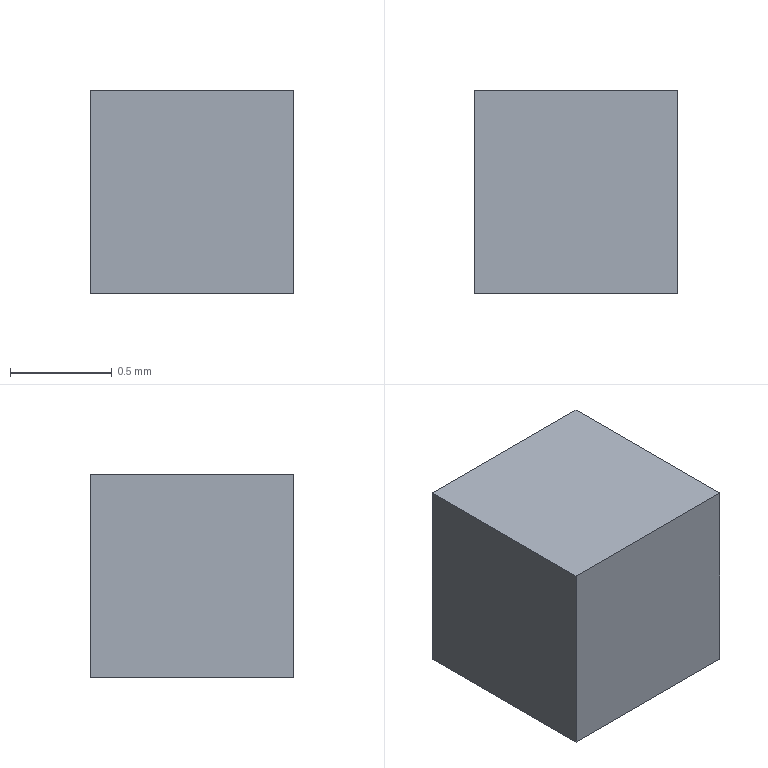Part | Creo | 1 solid | 6 faces | box 1 x 1 x 1 mm | volume 1 mm3 | plane 6
STEP:
#1=CARTESIAN_POINT('',(0.,0.,0.));
#2=DIRECTION('',(0.,0.,1.));
#3=DIRECTION('',(1.,0.,0.));
#4=AXIS2_PLACEMENT_3D('',#1,#2,#3);
#5=CARTESIAN_POINT('',(-0.5,-0.5,0.));
#6=VERTEX_POINT('',#5);
#7=CARTESIAN_POINT('',(0.5,-0.5,0.));
#8=VERTEX_POINT('',#7);
#9=CARTESIAN_POINT('',(-0.5,-0.5,0.));
#10=DIRECTION('',(1.,0.,0.));
#11=VECTOR('',#10,1.);
#12=LINE('',#9,#11);
#13=EDGE_CURVE('',#6,#8,#12,.T.);
#14=ORIENTED_EDGE('',*,*,#13,.T.);
#15=CARTESIAN_POINT('',(0.5,0.5,0.));
#16=VERTEX_POINT('',#15);
#17=CARTESIAN_POINT('',(0.5,-0.5,0.));
#18=DIRECTION('',(0.,1.,0.));
#19=VECTOR('',#18,1.);
#20=LINE('',#17,#19);
#21=EDGE_CURVE('',#8,#16,#20,.T.);
#22=ORIENTED_EDGE('',*,*,#21,.T.);
#23=CARTESIAN_POINT('',(-0.5,0.5,0.));
#24=VERTEX_POINT('',#23);
#25=CARTESIAN_POINT('',(0.5,0.5,0.));
#26=DIRECTION('',(-1.,0.,0.));
#27=VECTOR('',#26,1.);
#28=LINE('',#25,#27);
#29=EDGE_CURVE('',#16,#24,#28,.T.);
#30=ORIENTED_EDGE('',*,*,#29,.T.);
#31=CARTESIAN_POINT('',(-0.5,0.5,0.));
#32=DIRECTION('',(0.,-1.,0.));
#33=VECTOR('',#32,1.);
#34=LINE('',#31,#33);
#35=EDGE_CURVE('',#24,#6,#34,.T.);
#36=ORIENTED_EDGE('',*,*,#35,.T.);
#37=EDGE_LOOP('',(#14,#22,#30,#36));
#38=FACE_OUTER_BOUND('',#37,.F.);
#39=CARTESIAN_POINT('',(0.,0.,0.));
#40=DIRECTION('',(0.,0.,1.));
#41=DIRECTION('',(1.,0.,0.));
#42=AXIS2_PLACEMENT_3D('',#39,#40,#41);
#43=PLANE('',#42);
#44=ADVANCED_FACE('',(#38),#43,.F.);
#45=ORIENTED_EDGE('',*,*,#13,.F.);
#46=CARTESIAN_POINT('',(-0.5,-0.5,1.));
#47=VERTEX_POINT('',#46);
#48=CARTESIAN_POINT('',(-0.5,-0.5,0.));
#49=DIRECTION('',(0.,0.,1.));
#50=VECTOR('',#49,1.);
#51=LINE('',#48,#50);
#52=EDGE_CURVE('',#6,#47,#51,.T.);
#53=ORIENTED_EDGE('',*,*,#52,.T.);
#54=CARTESIAN_POINT('',(0.5,-0.5,1.));
#55=VERTEX_POINT('',#54);
#56=CARTESIAN_POINT('',(-0.5,-0.5,1.));
#57=DIRECTION('',(1.,0.,0.));
#58=VECTOR('',#57,1.);
#59=LINE('',#56,#58);
#60=EDGE_CURVE('',#47,#55,#59,.T.);
#61=ORIENTED_EDGE('',*,*,#60,.T.);
#62=CARTESIAN_POINT('',(0.5,-0.5,0.));
#63=DIRECTION('',(0.,0.,1.));
#64=VECTOR('',#63,1.);
#65=LINE('',#62,#64);
#66=EDGE_CURVE('',#8,#55,#65,.T.);
#67=ORIENTED_EDGE('',*,*,#66,.F.);
#68=EDGE_LOOP('',(#45,#53,#61,#67));
#69=FACE_OUTER_BOUND('',#68,.F.);
#70=CARTESIAN_POINT('',(-0.5,-0.5,0.));
#71=DIRECTION('',(0.,-1.,0.));
#72=DIRECTION('',(1.,0.,0.));
#73=AXIS2_PLACEMENT_3D('',#70,#71,#72);
#74=PLANE('',#73);
#75=ADVANCED_FACE('',(#69),#74,.T.);
#76=ORIENTED_EDGE('',*,*,#35,.F.);
#77=CARTESIAN_POINT('',(-0.5,0.5,1.));
#78=VERTEX_POINT('',#77);
#79=CARTESIAN_POINT('',(-0.5,0.5,0.));
#80=DIRECTION('',(0.,0.,1.));
#81=VECTOR('',#80,1.);
#82=LINE('',#79,#81);
#83=EDGE_CURVE('',#24,#78,#82,.T.);
#84=ORIENTED_EDGE('',*,*,#83,.T.);
#85=CARTESIAN_POINT('',(-0.5,0.5,1.));
#86=DIRECTION('',(0.,-1.,0.));
#87=VECTOR('',#86,1.);
#88=LINE('',#85,#87);
#89=EDGE_CURVE('',#78,#47,#88,.T.);
#90=ORIENTED_EDGE('',*,*,#89,.T.);
#91=ORIENTED_EDGE('',*,*,#52,.F.);
#92=EDGE_LOOP('',(#76,#84,#90,#91));
#93=FACE_OUTER_BOUND('',#92,.F.);
#94=CARTESIAN_POINT('',(-0.5,0.5,0.));
#95=DIRECTION('',(-1.,0.,0.));
#96=DIRECTION('',(0.,-1.,0.));
#97=AXIS2_PLACEMENT_3D('',#94,#95,#96);
#98=PLANE('',#97);
#99=ADVANCED_FACE('',(#93),#98,.T.);
#100=ORIENTED_EDGE('',*,*,#29,.F.);
#101=CARTESIAN_POINT('',(0.5,0.5,1.));
#102=VERTEX_POINT('',#101);
#103=CARTESIAN_POINT('',(0.5,0.5,0.));
#104=DIRECTION('',(0.,0.,1.));
#105=VECTOR('',#104,1.);
#106=LINE('',#103,#105);
#107=EDGE_CURVE('',#16,#102,#106,.T.);
#108=ORIENTED_EDGE('',*,*,#107,.T.);
#109=CARTESIAN_POINT('',(0.5,0.5,1.));
#110=DIRECTION('',(-1.,0.,0.));
#111=VECTOR('',#110,1.);
#112=LINE('',#109,#111);
#113=EDGE_CURVE('',#102,#78,#112,.T.);
#114=ORIENTED_EDGE('',*,*,#113,.T.);
#115=ORIENTED_EDGE('',*,*,#83,.F.);
#116=EDGE_LOOP('',(#100,#108,#114,#115));
#117=FACE_OUTER_BOUND('',#116,.F.);
#118=CARTESIAN_POINT('',(0.5,0.5,0.));
#119=DIRECTION('',(0.,1.,0.));
#120=DIRECTION('',(-1.,0.,0.));
#121=AXIS2_PLACEMENT_3D('',#118,#119,#120);
#122=PLANE('',#121);
#123=ADVANCED_FACE('',(#117),#122,.T.);
#124=ORIENTED_EDGE('',*,*,#21,.F.);
#125=ORIENTED_EDGE('',*,*,#66,.T.);
#126=CARTESIAN_POINT('',(0.5,-0.5,1.));
#127=DIRECTION('',(0.,1.,0.));
#128=VECTOR('',#127,1.);
#129=LINE('',#126,#128);
#130=EDGE_CURVE('',#55,#102,#129,.T.);
#131=ORIENTED_EDGE('',*,*,#130,.T.);
#132=ORIENTED_EDGE('',*,*,#107,.F.);
#133=EDGE_LOOP('',(#124,#125,#131,#132));
#134=FACE_OUTER_BOUND('',#133,.F.);
#135=CARTESIAN_POINT('',(0.5,-0.5,0.));
#136=DIRECTION('',(1.,0.,0.));
#137=DIRECTION('',(0.,1.,0.));
#138=AXIS2_PLACEMENT_3D('',#135,#136,#137);
#139=PLANE('',#138);
#140=ADVANCED_FACE('',(#134),#139,.T.);
#141=ORIENTED_EDGE('',*,*,#60,.F.);
#142=ORIENTED_EDGE('',*,*,#89,.F.);
#143=ORIENTED_EDGE('',*,*,#113,.F.);
#144=ORIENTED_EDGE('',*,*,#130,.F.);
#145=EDGE_LOOP('',(#141,#142,#143,#144));
#146=FACE_OUTER_BOUND('',#145,.F.);
#147=CARTESIAN_POINT('',(0.,0.,1.));
#148=DIRECTION('',(0.,0.,1.));
#149=DIRECTION('',(1.,0.,0.));
#150=AXIS2_PLACEMENT_3D('',#147,#148,#149);
#151=PLANE('',#150);
#152=ADVANCED_FACE('',(#146),#151,.T.);
#153=CLOSED_SHELL('',(#44,#75,#99,#123,#140,#152));
#154=MANIFOLD_SOLID_BREP('',#153);
#155=(LENGTH_UNIT()NAMED_UNIT(*)SI_UNIT(.MILLI.,.METRE.));
#156=UNCERTAINTY_MEASURE_WITH_UNIT(LENGTH_MEASURE(0.0001732),#155,'','');
#157=(NAMED_UNIT(*)PLANE_ANGLE_UNIT()SI_UNIT($,.RADIAN.));
#158=PLANE_ANGLE_MEASURE_WITH_UNIT(PLANE_ANGLE_MEASURE(0.01745),#157);
#159=(CONVERSION_BASED_UNIT('DEGREE',#158)NAMED_UNIT(*)PLANE_ANGLE_UNIT());
#160=(NAMED_UNIT(*)SI_UNIT($,.STERADIAN.)SOLID_ANGLE_UNIT());
#161=(GEOMETRIC_REPRESENTATION_CONTEXT(3)GLOBAL_UNCERTAINTY_ASSIGNED_CONTEXT((#156))GLOBAL_UNIT_ASSIGNED_CONTEXT((#155,#159,#160))REPRESENTATION_CONTEXT('',''));
#162=ADVANCED_BREP_SHAPE_REPRESENTATION('',(#4,#154),#161);